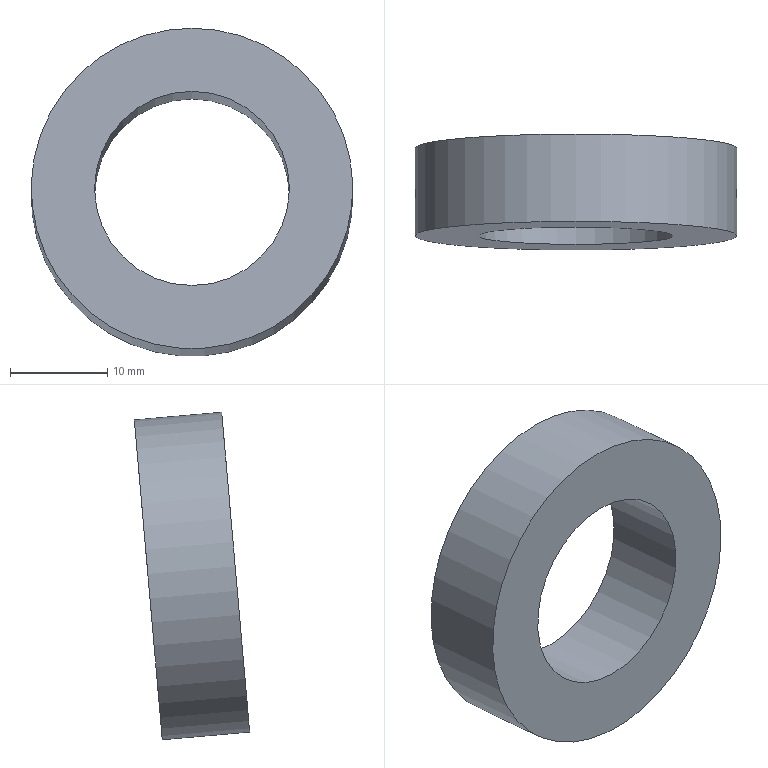Part | NX | features solid 2 | 1 solid | 4 faces | box 33 x 11.842 x 33.659 mm | volume 4870 mm3 | cylinder 2 | plane 2 | commonest cylinder face diameters 20 x1 33 x1
STEP:
#1=CARTESIAN_POINT('',(398.525,-66.07,-23.287));
#2=VERTEX_POINT('',#1);
#3=CARTESIAN_POINT('',(398.525,-67.508,-39.724));
#4=DIRECTION('',(0.,0.9962,-0.08716));
#5=DIRECTION('',(0.,0.08716,0.9962));
#6=AXIS2_PLACEMENT_3D('',#3,#4,#5);
#7=CIRCLE('',#6,16.5);
#8=EDGE_CURVE('',#2,#2,#7,.F.);
#9=ORIENTED_EDGE('',*,*,#8,.T.);
#10=EDGE_LOOP('',(#9));
#11=FACE_BOUND('',#10,.T.);
#12=CARTESIAN_POINT('',(398.525,-75.036,-22.502));
#13=VERTEX_POINT('',#12);
#14=CARTESIAN_POINT('',(398.525,-76.474,-38.939));
#15=DIRECTION('',(0.,0.9962,-0.08716));
#16=DIRECTION('',(0.,0.08716,0.9962));
#17=AXIS2_PLACEMENT_3D('',#14,#15,#16);
#18=CIRCLE('',#17,16.5);
#19=EDGE_CURVE('',#13,#13,#18,.F.);
#20=ORIENTED_EDGE('',*,*,#19,.F.);
#21=EDGE_LOOP('',(#20));
#22=FACE_BOUND('',#21,.T.);
#23=CARTESIAN_POINT('',(398.525,-67.508,-39.724));
#24=DIRECTION('',(0.,-0.9962,0.08716));
#25=DIRECTION('',(0.,-0.08716,-0.9962));
#26=AXIS2_PLACEMENT_3D('',#23,#24,#25);
#27=CYLINDRICAL_SURFACE('',#26,16.5);
#28=ADVANCED_FACE('',(#11,#22),#27,.T.);
#29=CARTESIAN_POINT('',(398.525,-66.636,-29.762));
#30=VERTEX_POINT('',#29);
#31=CARTESIAN_POINT('',(398.525,-67.508,-39.724));
#32=DIRECTION('',(0.,0.9962,-0.08716));
#33=DIRECTION('',(0.,0.08716,0.9962));
#34=AXIS2_PLACEMENT_3D('',#31,#32,#33);
#35=CIRCLE('',#34,10.);
#36=EDGE_CURVE('',#30,#30,#35,.F.);
#37=ORIENTED_EDGE('',*,*,#36,.F.);
#38=EDGE_LOOP('',(#37));
#39=FACE_BOUND('',#38,.T.);
#40=CARTESIAN_POINT('',(398.525,-75.602,-28.977));
#41=VERTEX_POINT('',#40);
#42=CARTESIAN_POINT('',(398.525,-76.474,-38.939));
#43=DIRECTION('',(0.,0.9962,-0.08716));
#44=DIRECTION('',(0.,0.08716,0.9962));
#45=AXIS2_PLACEMENT_3D('',#42,#43,#44);
#46=CIRCLE('',#45,10.);
#47=EDGE_CURVE('',#41,#41,#46,.F.);
#48=ORIENTED_EDGE('',*,*,#47,.T.);
#49=EDGE_LOOP('',(#48));
#50=FACE_BOUND('',#49,.T.);
#51=CARTESIAN_POINT('',(398.525,-67.508,-39.724));
#52=DIRECTION('',(0.,-0.9962,0.08716));
#53=DIRECTION('',(0.,-0.08716,-0.9962));
#54=AXIS2_PLACEMENT_3D('',#51,#52,#53);
#55=CYLINDRICAL_SURFACE('',#54,10.);
#56=ADVANCED_FACE('',(#39,#50),#55,.F.);
#57=ORIENTED_EDGE('',*,*,#8,.F.);
#58=EDGE_LOOP('',(#57));
#59=FACE_BOUND('',#58,.T.);
#60=ORIENTED_EDGE('',*,*,#36,.T.);
#61=EDGE_LOOP('',(#60));
#62=FACE_BOUND('',#61,.T.);
#63=CARTESIAN_POINT('',(398.525,-67.508,-39.724));
#64=DIRECTION('',(0.,0.9962,-0.08716));
#65=DIRECTION('',(-1.,0.,0.));
#66=AXIS2_PLACEMENT_3D('',#63,#64,#65);
#67=PLANE('',#66);
#68=ADVANCED_FACE('',(#59,#62),#67,.T.);
#69=ORIENTED_EDGE('',*,*,#19,.T.);
#70=EDGE_LOOP('',(#69));
#71=FACE_BOUND('',#70,.T.);
#72=ORIENTED_EDGE('',*,*,#47,.F.);
#73=EDGE_LOOP('',(#72));
#74=FACE_BOUND('',#73,.T.);
#75=CARTESIAN_POINT('',(398.525,-76.474,-38.939));
#76=DIRECTION('',(0.,0.9962,-0.08716));
#77=DIRECTION('',(-1.,0.,0.));
#78=AXIS2_PLACEMENT_3D('',#75,#76,#77);
#79=PLANE('',#78);
#80=ADVANCED_FACE('',(#71,#74),#79,.F.);
#81=CLOSED_SHELL('',(#28,#56,#68,#80));
#82=MANIFOLD_SOLID_BREP('',#81);
#83=(LENGTH_UNIT()NAMED_UNIT(*)SI_UNIT(.MILLI.,.METRE.));
#84=UNCERTAINTY_MEASURE_WITH_UNIT(LENGTH_MEASURE(0.00001),#83,'','');
#85=(NAMED_UNIT(*)PLANE_ANGLE_UNIT()SI_UNIT($,.RADIAN.));
#86=(NAMED_UNIT(*)SI_UNIT($,.STERADIAN.)SOLID_ANGLE_UNIT());
#87=(GEOMETRIC_REPRESENTATION_CONTEXT(3)GLOBAL_UNCERTAINTY_ASSIGNED_CONTEXT((#84))GLOBAL_UNIT_ASSIGNED_CONTEXT((#83,#85,#86))REPRESENTATION_CONTEXT('',''));
#88=ADVANCED_BREP_SHAPE_REPRESENTATION('',(#82),#87);